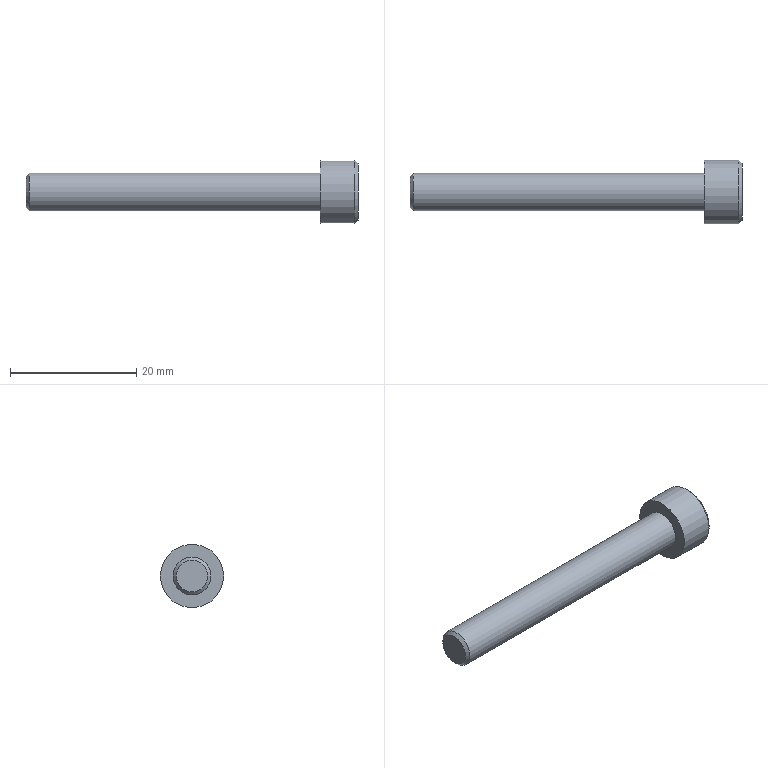Part | STEP file | solid 150 | 1 solid | 14 faces | box 52.5 x 10 x 10 mm | volume 1715 mm3 | plane 10 | cone 2 | cylinder 2 | commonest cylinder face diameters 6 x1 10 x1